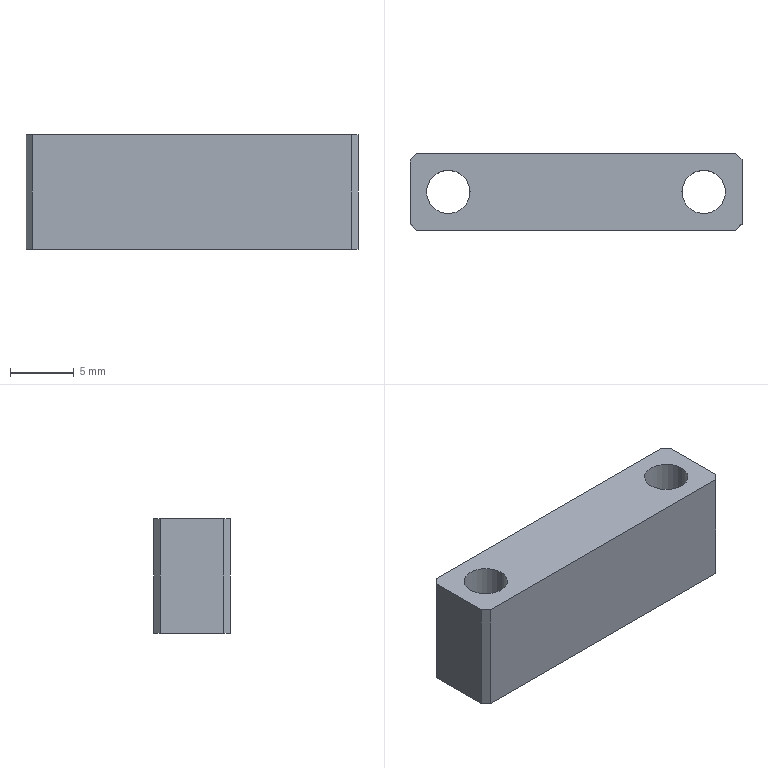Part | SolidWorks | features Chamfer 1, Extrusion 1, HoleWzd 1 | 1 solid | 14 faces | box 26 x 6 x 9 mm | volume 1236 mm3 | plane 10 | cylinder 4 | commonest cylinder face diameters 3.4 x4
STEP:
#1=CARTESIAN_POINT('',(-11.7,0.,0.));
#2=VERTEX_POINT('',#1);
#3=CARTESIAN_POINT('',(-8.3,0.,0.));
#4=VERTEX_POINT('',#3);
#5=CARTESIAN_POINT('',(-10.,0.,0.));
#6=DIRECTION('',(0.,0.,1.));
#7=DIRECTION('',(1.,0.,0.));
#8=AXIS2_PLACEMENT_3D('',#5,#6,#7);
#9=CIRCLE('',#8,1.7);
#10=EDGE_CURVE('',#2,#4,#9,.T.);
#11=ORIENTED_EDGE('',*,*,#10,.F.);
#12=CARTESIAN_POINT('',(-11.7,0.,9.));
#13=VERTEX_POINT('',#12);
#14=CARTESIAN_POINT('',(-11.7,0.,9.));
#15=DIRECTION('',(0.,0.,1.));
#16=VECTOR('',#15,1000.);
#17=LINE('',#14,#16);
#18=EDGE_CURVE('',#2,#13,#17,.T.);
#19=ORIENTED_EDGE('',*,*,#18,.T.);
#20=CARTESIAN_POINT('',(-8.3,0.,9.));
#21=VERTEX_POINT('',#20);
#22=CARTESIAN_POINT('',(-10.,0.,9.));
#23=DIRECTION('',(0.,0.,1.));
#24=DIRECTION('',(1.,0.,0.));
#25=AXIS2_PLACEMENT_3D('',#22,#23,#24);
#26=CIRCLE('',#25,1.7);
#27=EDGE_CURVE('',#13,#21,#26,.T.);
#28=ORIENTED_EDGE('',*,*,#27,.T.);
#29=CARTESIAN_POINT('',(-8.3,0.,9.));
#30=DIRECTION('',(0.,0.,1.));
#31=VECTOR('',#30,1000.);
#32=LINE('',#29,#31);
#33=EDGE_CURVE('',#4,#21,#32,.T.);
#34=ORIENTED_EDGE('',*,*,#33,.F.);
#35=EDGE_LOOP('',(#11,#19,#28,#34));
#36=FACE_OUTER_BOUND('',#35,.T.);
#37=CARTESIAN_POINT('',(-10.,0.,9.));
#38=DIRECTION('',(0.,0.,1.));
#39=DIRECTION('',(1.,0.,0.));
#40=AXIS2_PLACEMENT_3D('',#37,#38,#39);
#41=CYLINDRICAL_SURFACE('',#40,1.7);
#42=ADVANCED_FACE('',(#36),#41,.F.);
#43=CARTESIAN_POINT('',(8.3,0.,0.));
#44=VERTEX_POINT('',#43);
#45=CARTESIAN_POINT('',(11.7,0.,0.));
#46=VERTEX_POINT('',#45);
#47=CARTESIAN_POINT('',(10.,0.,0.));
#48=DIRECTION('',(0.,0.,1.));
#49=DIRECTION('',(1.,0.,0.));
#50=AXIS2_PLACEMENT_3D('',#47,#48,#49);
#51=CIRCLE('',#50,1.7);
#52=EDGE_CURVE('',#44,#46,#51,.T.);
#53=ORIENTED_EDGE('',*,*,#52,.F.);
#54=CARTESIAN_POINT('',(8.3,0.,9.));
#55=VERTEX_POINT('',#54);
#56=CARTESIAN_POINT('',(8.3,0.,9.));
#57=DIRECTION('',(0.,0.,1.));
#58=VECTOR('',#57,1000.);
#59=LINE('',#56,#58);
#60=EDGE_CURVE('',#44,#55,#59,.T.);
#61=ORIENTED_EDGE('',*,*,#60,.T.);
#62=CARTESIAN_POINT('',(11.7,0.,9.));
#63=VERTEX_POINT('',#62);
#64=CARTESIAN_POINT('',(10.,0.,9.));
#65=DIRECTION('',(0.,0.,1.));
#66=DIRECTION('',(1.,0.,0.));
#67=AXIS2_PLACEMENT_3D('',#64,#65,#66);
#68=CIRCLE('',#67,1.7);
#69=EDGE_CURVE('',#55,#63,#68,.T.);
#70=ORIENTED_EDGE('',*,*,#69,.T.);
#71=CARTESIAN_POINT('',(11.7,0.,9.));
#72=DIRECTION('',(0.,0.,1.));
#73=VECTOR('',#72,1000.);
#74=LINE('',#71,#73);
#75=EDGE_CURVE('',#46,#63,#74,.T.);
#76=ORIENTED_EDGE('',*,*,#75,.F.);
#77=EDGE_LOOP('',(#53,#61,#70,#76));
#78=FACE_OUTER_BOUND('',#77,.T.);
#79=CARTESIAN_POINT('',(10.,0.,9.));
#80=DIRECTION('',(0.,0.,1.));
#81=DIRECTION('',(1.,0.,0.));
#82=AXIS2_PLACEMENT_3D('',#79,#80,#81);
#83=CYLINDRICAL_SURFACE('',#82,1.7);
#84=ADVANCED_FACE('',(#78),#83,.F.);
#85=CARTESIAN_POINT('',(13.,-2.5,0.));
#86=VERTEX_POINT('',#85);
#87=CARTESIAN_POINT('',(13.,2.5,0.));
#88=VERTEX_POINT('',#87);
#89=CARTESIAN_POINT('',(13.,3.,0.));
#90=DIRECTION('',(0.,1.,0.));
#91=VECTOR('',#90,1000.);
#92=LINE('',#89,#91);
#93=EDGE_CURVE('',#86,#88,#92,.T.);
#94=ORIENTED_EDGE('',*,*,#93,.T.);
#95=CARTESIAN_POINT('',(13.,2.5,9.));
#96=VERTEX_POINT('',#95);
#97=CARTESIAN_POINT('',(13.,2.5,9.));
#98=DIRECTION('',(0.,0.,1.));
#99=VECTOR('',#98,1000.);
#100=LINE('',#97,#99);
#101=EDGE_CURVE('',#88,#96,#100,.T.);
#102=ORIENTED_EDGE('',*,*,#101,.T.);
#103=CARTESIAN_POINT('',(13.,-2.5,9.));
#104=VERTEX_POINT('',#103);
#105=CARTESIAN_POINT('',(13.,3.,9.));
#106=DIRECTION('',(0.,1.,0.));
#107=VECTOR('',#106,1000.);
#108=LINE('',#105,#107);
#109=EDGE_CURVE('',#104,#96,#108,.T.);
#110=ORIENTED_EDGE('',*,*,#109,.F.);
#111=CARTESIAN_POINT('',(13.,-2.5,9.));
#112=DIRECTION('',(0.,0.,-1.));
#113=VECTOR('',#112,1000.);
#114=LINE('',#111,#113);
#115=EDGE_CURVE('',#104,#86,#114,.T.);
#116=ORIENTED_EDGE('',*,*,#115,.T.);
#117=EDGE_LOOP('',(#94,#102,#110,#116));
#118=FACE_OUTER_BOUND('',#117,.T.);
#119=CARTESIAN_POINT('',(13.,3.,9.));
#120=DIRECTION('',(-1.,0.,0.));
#121=DIRECTION('',(0.,0.,1.));
#122=AXIS2_PLACEMENT_3D('',#119,#120,#121);
#123=PLANE('',#122);
#124=ADVANCED_FACE('',(#118),#123,.F.);
#125=CARTESIAN_POINT('',(12.5,3.,9.));
#126=VERTEX_POINT('',#125);
#127=CARTESIAN_POINT('',(-12.5,3.,9.));
#128=VERTEX_POINT('',#127);
#129=CARTESIAN_POINT('',(-13.,3.,9.));
#130=DIRECTION('',(-1.,0.,0.));
#131=VECTOR('',#130,1000.);
#132=LINE('',#129,#131);
#133=EDGE_CURVE('',#126,#128,#132,.T.);
#134=ORIENTED_EDGE('',*,*,#133,.F.);
#135=CARTESIAN_POINT('',(12.5,3.,0.));
#136=VERTEX_POINT('',#135);
#137=CARTESIAN_POINT('',(12.5,3.,9.));
#138=DIRECTION('',(0.,0.,-1.));
#139=VECTOR('',#138,1000.);
#140=LINE('',#137,#139);
#141=EDGE_CURVE('',#126,#136,#140,.T.);
#142=ORIENTED_EDGE('',*,*,#141,.T.);
#143=CARTESIAN_POINT('',(-12.5,3.,0.));
#144=VERTEX_POINT('',#143);
#145=CARTESIAN_POINT('',(-13.,3.,0.));
#146=DIRECTION('',(-1.,0.,0.));
#147=VECTOR('',#146,1000.);
#148=LINE('',#145,#147);
#149=EDGE_CURVE('',#136,#144,#148,.T.);
#150=ORIENTED_EDGE('',*,*,#149,.T.);
#151=CARTESIAN_POINT('',(-12.5,3.,9.));
#152=DIRECTION('',(0.,0.,1.));
#153=VECTOR('',#152,1000.);
#154=LINE('',#151,#153);
#155=EDGE_CURVE('',#144,#128,#154,.T.);
#156=ORIENTED_EDGE('',*,*,#155,.T.);
#157=EDGE_LOOP('',(#134,#142,#150,#156));
#158=FACE_OUTER_BOUND('',#157,.T.);
#159=CARTESIAN_POINT('',(-13.,3.,9.));
#160=DIRECTION('',(0.,-1.,0.));
#161=DIRECTION('',(0.,0.,-1.));
#162=AXIS2_PLACEMENT_3D('',#159,#160,#161);
#163=PLANE('',#162);
#164=ADVANCED_FACE('',(#158),#163,.F.);
#165=CARTESIAN_POINT('',(-13.,2.5,9.));
#166=VERTEX_POINT('',#165);
#167=CARTESIAN_POINT('',(-13.,-2.5,9.));
#168=VERTEX_POINT('',#167);
#169=CARTESIAN_POINT('',(-13.,3.,9.));
#170=DIRECTION('',(0.,-1.,0.));
#171=VECTOR('',#170,1000.);
#172=LINE('',#169,#171);
#173=EDGE_CURVE('',#166,#168,#172,.T.);
#174=ORIENTED_EDGE('',*,*,#173,.F.);
#175=CARTESIAN_POINT('',(-13.,2.5,0.));
#176=VERTEX_POINT('',#175);
#177=CARTESIAN_POINT('',(-13.,2.5,9.));
#178=DIRECTION('',(0.,0.,-1.));
#179=VECTOR('',#178,1000.);
#180=LINE('',#177,#179);
#181=EDGE_CURVE('',#166,#176,#180,.T.);
#182=ORIENTED_EDGE('',*,*,#181,.T.);
#183=CARTESIAN_POINT('',(-13.,-2.5,0.));
#184=VERTEX_POINT('',#183);
#185=CARTESIAN_POINT('',(-13.,3.,0.));
#186=DIRECTION('',(0.,-1.,0.));
#187=VECTOR('',#186,1000.);
#188=LINE('',#185,#187);
#189=EDGE_CURVE('',#176,#184,#188,.T.);
#190=ORIENTED_EDGE('',*,*,#189,.T.);
#191=CARTESIAN_POINT('',(-13.,-2.5,9.));
#192=DIRECTION('',(0.,0.,1.));
#193=VECTOR('',#192,1000.);
#194=LINE('',#191,#193);
#195=EDGE_CURVE('',#184,#168,#194,.T.);
#196=ORIENTED_EDGE('',*,*,#195,.T.);
#197=EDGE_LOOP('',(#174,#182,#190,#196));
#198=FACE_OUTER_BOUND('',#197,.T.);
#199=CARTESIAN_POINT('',(-13.,3.,9.));
#200=DIRECTION('',(1.,0.,0.));
#201=DIRECTION('',(0.,0.,-1.));
#202=AXIS2_PLACEMENT_3D('',#199,#200,#201);
#203=PLANE('',#202);
#204=ADVANCED_FACE('',(#198),#203,.F.);
#205=CARTESIAN_POINT('',(-12.5,-3.,0.));
#206=VERTEX_POINT('',#205);
#207=CARTESIAN_POINT('',(12.5,-3.,0.));
#208=VERTEX_POINT('',#207);
#209=CARTESIAN_POINT('',(-13.,-3.,0.));
#210=DIRECTION('',(1.,0.,0.));
#211=VECTOR('',#210,1000.);
#212=LINE('',#209,#211);
#213=EDGE_CURVE('',#206,#208,#212,.T.);
#214=ORIENTED_EDGE('',*,*,#213,.T.);
#215=CARTESIAN_POINT('',(12.5,-3.,9.));
#216=VERTEX_POINT('',#215);
#217=CARTESIAN_POINT('',(12.5,-3.,9.));
#218=DIRECTION('',(0.,0.,1.));
#219=VECTOR('',#218,1000.);
#220=LINE('',#217,#219);
#221=EDGE_CURVE('',#208,#216,#220,.T.);
#222=ORIENTED_EDGE('',*,*,#221,.T.);
#223=CARTESIAN_POINT('',(-12.5,-3.,9.));
#224=VERTEX_POINT('',#223);
#225=CARTESIAN_POINT('',(-13.,-3.,9.));
#226=DIRECTION('',(1.,0.,0.));
#227=VECTOR('',#226,1000.);
#228=LINE('',#225,#227);
#229=EDGE_CURVE('',#224,#216,#228,.T.);
#230=ORIENTED_EDGE('',*,*,#229,.F.);
#231=CARTESIAN_POINT('',(-12.5,-3.,9.));
#232=DIRECTION('',(0.,0.,-1.));
#233=VECTOR('',#232,1000.);
#234=LINE('',#231,#233);
#235=EDGE_CURVE('',#224,#206,#234,.T.);
#236=ORIENTED_EDGE('',*,*,#235,.T.);
#237=EDGE_LOOP('',(#214,#222,#230,#236));
#238=FACE_OUTER_BOUND('',#237,.T.);
#239=CARTESIAN_POINT('',(-13.,-3.,9.));
#240=DIRECTION('',(0.,1.,0.));
#241=DIRECTION('',(0.,0.,1.));
#242=AXIS2_PLACEMENT_3D('',#239,#240,#241);
#243=PLANE('',#242);
#244=ADVANCED_FACE('',(#238),#243,.F.);
#245=CARTESIAN_POINT('',(-10.,0.,9.));
#246=DIRECTION('',(0.,0.,1.));
#247=DIRECTION('',(1.,0.,0.));
#248=AXIS2_PLACEMENT_3D('',#245,#246,#247);
#249=CIRCLE('',#248,1.7);
#250=EDGE_CURVE('',#21,#13,#249,.T.);
#251=ORIENTED_EDGE('',*,*,#250,.F.);
#252=ORIENTED_EDGE('',*,*,#27,.F.);
#253=EDGE_LOOP('',(#251,#252));
#254=FACE_BOUND('',#253,.T.);
#255=CARTESIAN_POINT('',(10.,0.,9.));
#256=DIRECTION('',(0.,0.,1.));
#257=DIRECTION('',(1.,0.,0.));
#258=AXIS2_PLACEMENT_3D('',#255,#256,#257);
#259=CIRCLE('',#258,1.7);
#260=EDGE_CURVE('',#63,#55,#259,.T.);
#261=ORIENTED_EDGE('',*,*,#260,.F.);
#262=ORIENTED_EDGE('',*,*,#69,.F.);
#263=EDGE_LOOP('',(#261,#262));
#264=FACE_BOUND('',#263,.T.);
#265=ORIENTED_EDGE('',*,*,#109,.T.);
#266=CARTESIAN_POINT('',(15.75,-0.25,9.));
#267=DIRECTION('',(-0.7071,0.7071,0.));
#268=VECTOR('',#267,1000.);
#269=LINE('',#266,#268);
#270=EDGE_CURVE('',#96,#126,#269,.T.);
#271=ORIENTED_EDGE('',*,*,#270,.T.);
#272=ORIENTED_EDGE('',*,*,#133,.T.);
#273=CARTESIAN_POINT('',(-2.75,12.75,9.));
#274=DIRECTION('',(-0.7071,-0.7071,0.));
#275=VECTOR('',#274,1000.);
#276=LINE('',#273,#275);
#277=EDGE_CURVE('',#128,#166,#276,.T.);
#278=ORIENTED_EDGE('',*,*,#277,.T.);
#279=ORIENTED_EDGE('',*,*,#173,.T.);
#280=CARTESIAN_POINT('',(0.25,-15.75,9.));
#281=DIRECTION('',(0.7071,-0.7071,0.));
#282=VECTOR('',#281,1000.);
#283=LINE('',#280,#282);
#284=EDGE_CURVE('',#168,#224,#283,.T.);
#285=ORIENTED_EDGE('',*,*,#284,.T.);
#286=ORIENTED_EDGE('',*,*,#229,.T.);
#287=CARTESIAN_POINT('',(12.75,-2.75,9.));
#288=DIRECTION('',(0.7071,0.7071,0.));
#289=VECTOR('',#288,1000.);
#290=LINE('',#287,#289);
#291=EDGE_CURVE('',#216,#104,#290,.T.);
#292=ORIENTED_EDGE('',*,*,#291,.T.);
#293=EDGE_LOOP('',(#265,#271,#272,#278,#279,#285,#286,#292));
#294=FACE_OUTER_BOUND('',#293,.T.);
#295=CARTESIAN_POINT('',(13.,-3.,9.));
#296=DIRECTION('',(0.,0.,1.));
#297=DIRECTION('',(1.,0.,0.));
#298=AXIS2_PLACEMENT_3D('',#295,#296,#297);
#299=PLANE('',#298);
#300=ADVANCED_FACE('',(#254,#264,#294),#299,.T.);
#301=CARTESIAN_POINT('',(-10.,0.,0.));
#302=DIRECTION('',(0.,0.,1.));
#303=DIRECTION('',(1.,0.,0.));
#304=AXIS2_PLACEMENT_3D('',#301,#302,#303);
#305=CIRCLE('',#304,1.7);
#306=EDGE_CURVE('',#4,#2,#305,.T.);
#307=ORIENTED_EDGE('',*,*,#306,.T.);
#308=ORIENTED_EDGE('',*,*,#10,.T.);
#309=EDGE_LOOP('',(#307,#308));
#310=FACE_BOUND('',#309,.T.);
#311=CARTESIAN_POINT('',(10.,0.,0.));
#312=DIRECTION('',(0.,0.,1.));
#313=DIRECTION('',(1.,0.,0.));
#314=AXIS2_PLACEMENT_3D('',#311,#312,#313);
#315=CIRCLE('',#314,1.7);
#316=EDGE_CURVE('',#46,#44,#315,.T.);
#317=ORIENTED_EDGE('',*,*,#316,.T.);
#318=ORIENTED_EDGE('',*,*,#52,.T.);
#319=EDGE_LOOP('',(#317,#318));
#320=FACE_BOUND('',#319,.T.);
#321=ORIENTED_EDGE('',*,*,#149,.F.);
#322=CARTESIAN_POINT('',(12.5,3.,0.));
#323=DIRECTION('',(0.7071,-0.7071,0.));
#324=VECTOR('',#323,1000.);
#325=LINE('',#322,#324);
#326=EDGE_CURVE('',#136,#88,#325,.T.);
#327=ORIENTED_EDGE('',*,*,#326,.T.);
#328=ORIENTED_EDGE('',*,*,#93,.F.);
#329=CARTESIAN_POINT('',(13.,-2.5,0.));
#330=DIRECTION('',(-0.7071,-0.7071,0.));
#331=VECTOR('',#330,1000.);
#332=LINE('',#329,#331);
#333=EDGE_CURVE('',#86,#208,#332,.T.);
#334=ORIENTED_EDGE('',*,*,#333,.T.);
#335=ORIENTED_EDGE('',*,*,#213,.F.);
#336=CARTESIAN_POINT('',(-12.5,-3.,0.));
#337=DIRECTION('',(-0.7071,0.7071,0.));
#338=VECTOR('',#337,1000.);
#339=LINE('',#336,#338);
#340=EDGE_CURVE('',#206,#184,#339,.T.);
#341=ORIENTED_EDGE('',*,*,#340,.T.);
#342=ORIENTED_EDGE('',*,*,#189,.F.);
#343=CARTESIAN_POINT('',(-13.,2.5,0.));
#344=DIRECTION('',(0.7071,0.7071,0.));
#345=VECTOR('',#344,1000.);
#346=LINE('',#343,#345);
#347=EDGE_CURVE('',#176,#144,#346,.T.);
#348=ORIENTED_EDGE('',*,*,#347,.T.);
#349=EDGE_LOOP('',(#321,#327,#328,#334,#335,#341,#342,#348));
#350=FACE_OUTER_BOUND('',#349,.T.);
#351=CARTESIAN_POINT('',(13.,-3.,0.));
#352=DIRECTION('',(0.,0.,1.));
#353=DIRECTION('',(1.,0.,0.));
#354=AXIS2_PLACEMENT_3D('',#351,#352,#353);
#355=PLANE('',#354);
#356=ADVANCED_FACE('',(#310,#320,#350),#355,.F.);
#357=ORIENTED_EDGE('',*,*,#60,.F.);
#358=ORIENTED_EDGE('',*,*,#316,.F.);
#359=ORIENTED_EDGE('',*,*,#75,.T.);
#360=ORIENTED_EDGE('',*,*,#260,.T.);
#361=EDGE_LOOP('',(#357,#358,#359,#360));
#362=FACE_OUTER_BOUND('',#361,.T.);
#363=CARTESIAN_POINT('',(10.,0.,9.));
#364=DIRECTION('',(0.,0.,1.));
#365=DIRECTION('',(1.,0.,0.));
#366=AXIS2_PLACEMENT_3D('',#363,#364,#365);
#367=CYLINDRICAL_SURFACE('',#366,1.7);
#368=ADVANCED_FACE('',(#362),#367,.F.);
#369=ORIENTED_EDGE('',*,*,#18,.F.);
#370=ORIENTED_EDGE('',*,*,#306,.F.);
#371=ORIENTED_EDGE('',*,*,#33,.T.);
#372=ORIENTED_EDGE('',*,*,#250,.T.);
#373=EDGE_LOOP('',(#369,#370,#371,#372));
#374=FACE_OUTER_BOUND('',#373,.T.);
#375=CARTESIAN_POINT('',(-10.,0.,9.));
#376=DIRECTION('',(0.,0.,1.));
#377=DIRECTION('',(1.,0.,0.));
#378=AXIS2_PLACEMENT_3D('',#375,#376,#377);
#379=CYLINDRICAL_SURFACE('',#378,1.7);
#380=ADVANCED_FACE('',(#374),#379,.F.);
#381=ORIENTED_EDGE('',*,*,#270,.F.);
#382=ORIENTED_EDGE('',*,*,#101,.F.);
#383=ORIENTED_EDGE('',*,*,#326,.F.);
#384=ORIENTED_EDGE('',*,*,#141,.F.);
#385=EDGE_LOOP('',(#381,#382,#383,#384));
#386=FACE_OUTER_BOUND('',#385,.T.);
#387=CARTESIAN_POINT('',(12.5,3.,9.));
#388=DIRECTION('',(-0.7071,-0.7071,0.));
#389=DIRECTION('',(0.7071,-0.7071,0.));
#390=AXIS2_PLACEMENT_3D('',#387,#388,#389);
#391=PLANE('',#390);
#392=ADVANCED_FACE('',(#386),#391,.F.);
#393=ORIENTED_EDGE('',*,*,#291,.F.);
#394=ORIENTED_EDGE('',*,*,#221,.F.);
#395=ORIENTED_EDGE('',*,*,#333,.F.);
#396=ORIENTED_EDGE('',*,*,#115,.F.);
#397=EDGE_LOOP('',(#393,#394,#395,#396));
#398=FACE_OUTER_BOUND('',#397,.T.);
#399=CARTESIAN_POINT('',(13.,-2.5,9.));
#400=DIRECTION('',(-0.7071,0.7071,0.));
#401=DIRECTION('',(-0.7071,-0.7071,0.));
#402=AXIS2_PLACEMENT_3D('',#399,#400,#401);
#403=PLANE('',#402);
#404=ADVANCED_FACE('',(#398),#403,.F.);
#405=ORIENTED_EDGE('',*,*,#277,.F.);
#406=ORIENTED_EDGE('',*,*,#155,.F.);
#407=ORIENTED_EDGE('',*,*,#347,.F.);
#408=ORIENTED_EDGE('',*,*,#181,.F.);
#409=EDGE_LOOP('',(#405,#406,#407,#408));
#410=FACE_OUTER_BOUND('',#409,.T.);
#411=CARTESIAN_POINT('',(-13.,2.5,9.));
#412=DIRECTION('',(0.7071,-0.7071,0.));
#413=DIRECTION('',(0.7071,0.7071,0.));
#414=AXIS2_PLACEMENT_3D('',#411,#412,#413);
#415=PLANE('',#414);
#416=ADVANCED_FACE('',(#410),#415,.F.);
#417=ORIENTED_EDGE('',*,*,#284,.F.);
#418=ORIENTED_EDGE('',*,*,#195,.F.);
#419=ORIENTED_EDGE('',*,*,#340,.F.);
#420=ORIENTED_EDGE('',*,*,#235,.F.);
#421=EDGE_LOOP('',(#417,#418,#419,#420));
#422=FACE_OUTER_BOUND('',#421,.T.);
#423=CARTESIAN_POINT('',(-12.5,-3.,9.));
#424=DIRECTION('',(0.7071,0.7071,0.));
#425=DIRECTION('',(-0.7071,0.7071,0.));
#426=AXIS2_PLACEMENT_3D('',#423,#424,#425);
#427=PLANE('',#426);
#428=ADVANCED_FACE('',(#422),#427,.F.);
#429=CLOSED_SHELL('',(#42,#84,#124,#164,#204,#244,#300,#356,#368,#380,#392,#404,#416,#428));
#430=MANIFOLD_SOLID_BREP('',#429);
#431=CARTESIAN_POINT('',(0.,0.,0.));
#432=DIRECTION('',(0.,0.,1.));
#433=DIRECTION('',(1.,0.,0.));
#434=AXIS2_PLACEMENT_3D('',#431,#432,#433);
#435=(LENGTH_UNIT()NAMED_UNIT(*)SI_UNIT(.MILLI.,.METRE.));
#436=UNCERTAINTY_MEASURE_WITH_UNIT(LENGTH_MEASURE(0.00001),#435,'','');
#437=(NAMED_UNIT(*)PLANE_ANGLE_UNIT()SI_UNIT($,.RADIAN.));
#438=(NAMED_UNIT(*)SI_UNIT($,.STERADIAN.)SOLID_ANGLE_UNIT());
#439=(GEOMETRIC_REPRESENTATION_CONTEXT(3)GLOBAL_UNCERTAINTY_ASSIGNED_CONTEXT((#436))GLOBAL_UNIT_ASSIGNED_CONTEXT((#435,#437,#438))REPRESENTATION_CONTEXT('',''));
#440=ADVANCED_BREP_SHAPE_REPRESENTATION('',(#430,#434),#439);